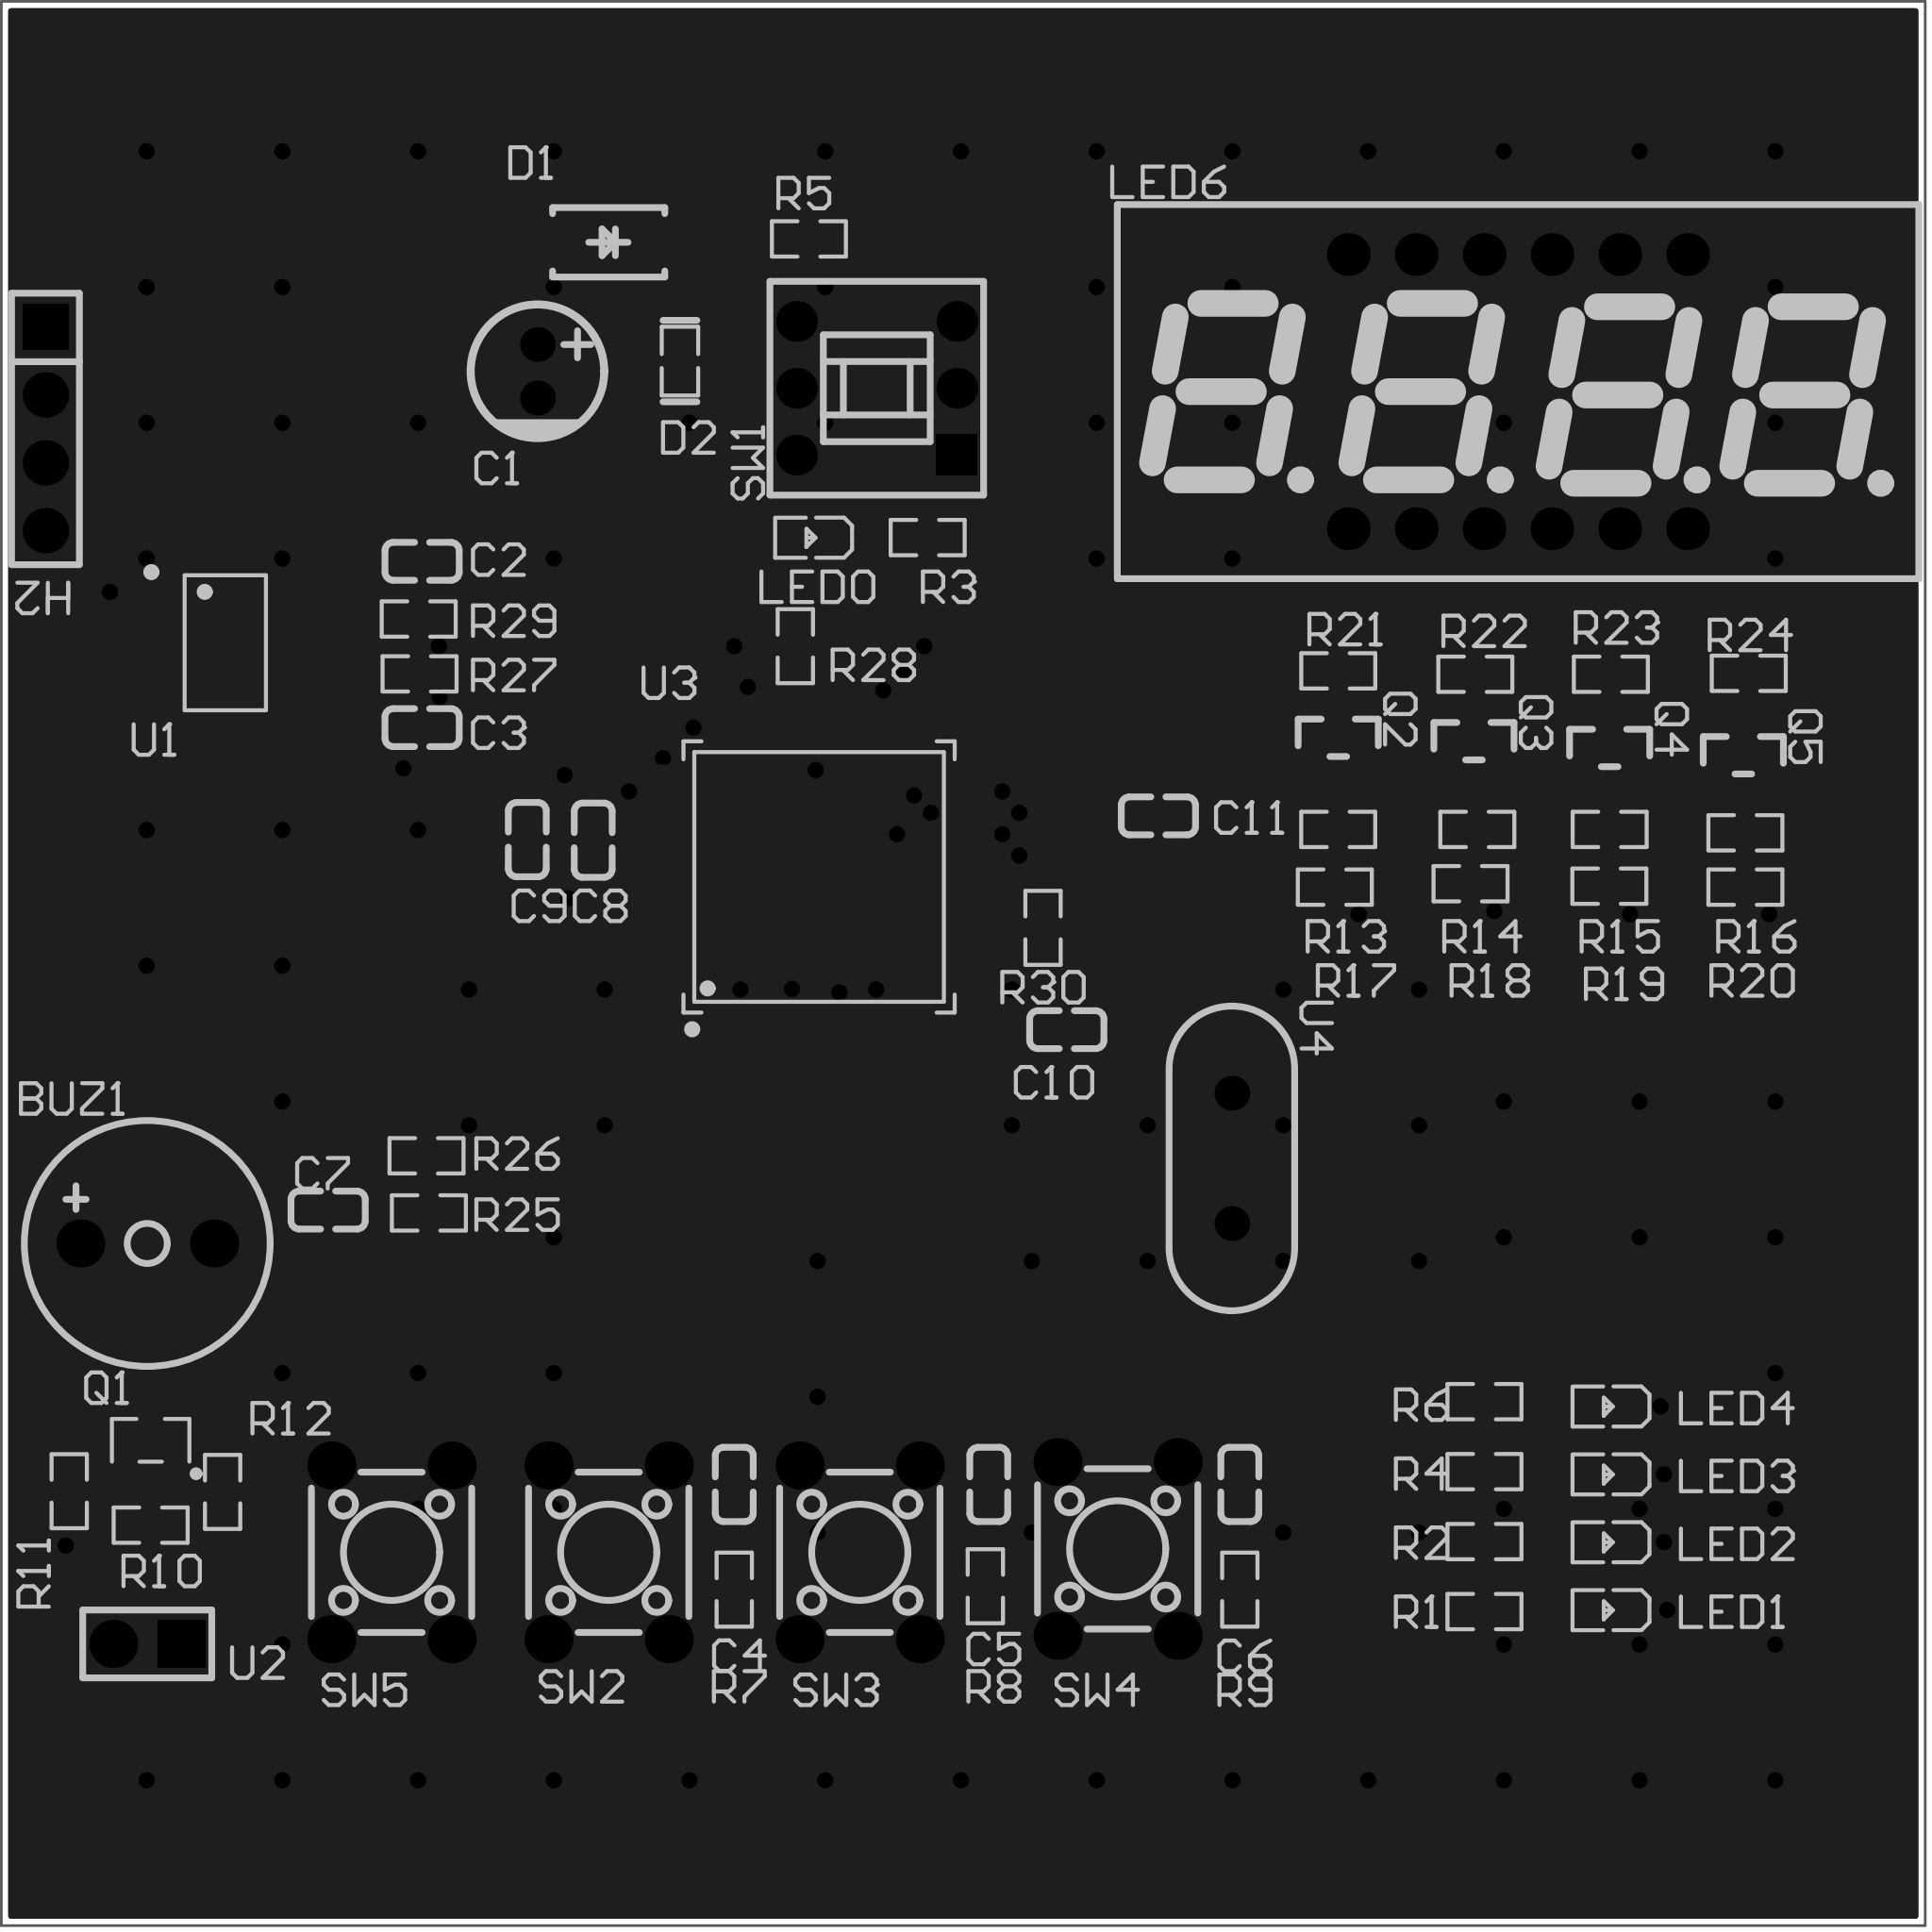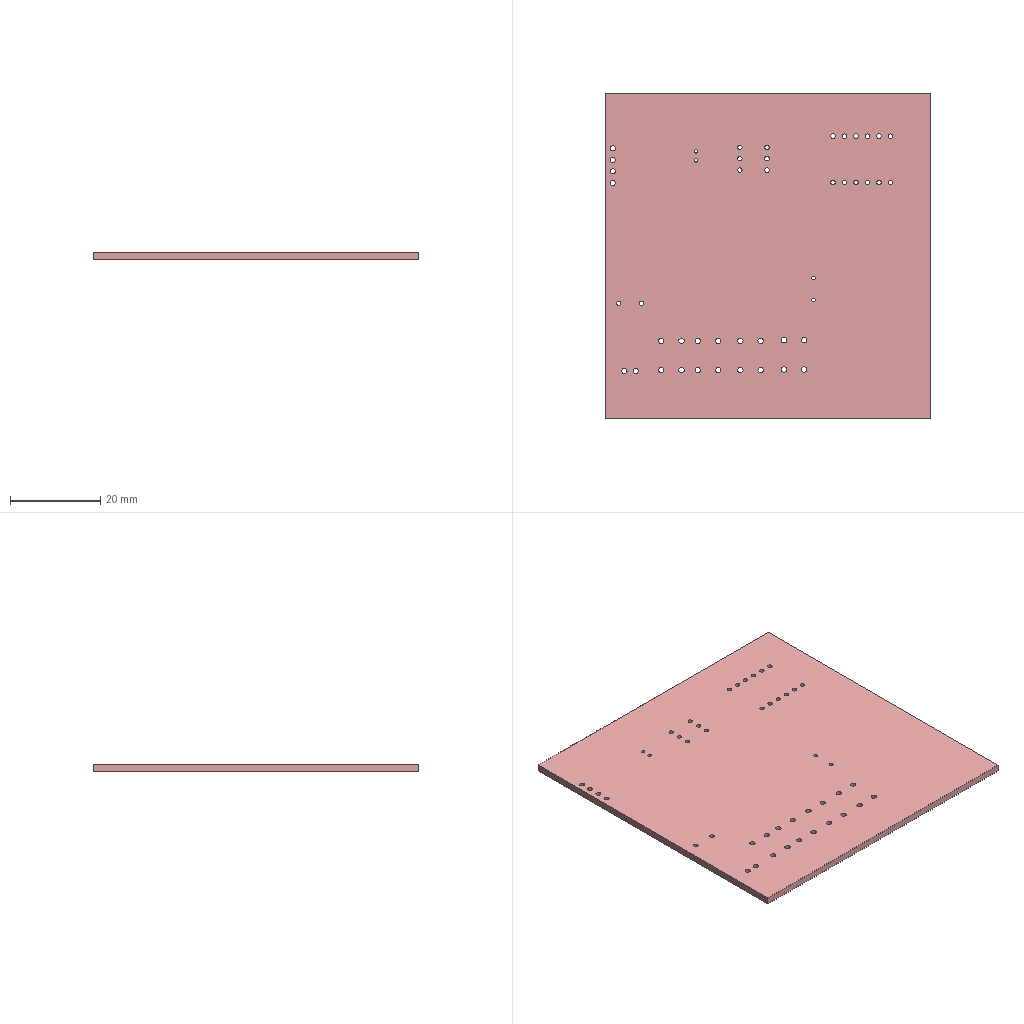Circuit board layout | Altium Designer | box 72 x 72 x 1.6 mm
Layer stack:
# Altium Designer layer stack of  (unit mm; dielectric type: 0 none, 1 core, 2 prepreg, 3 surface material)
index,name,kind,layer,copper_thickness_mm,dielectric_type,dielectric_thickness_mm,dielectric_material,dielectric_constant
0,Top Paste Mask Layer,other,,,,,,
1,Top Silkscreen Layer,other,,,,,,
2,Top Solder Mask Layer,dielectric,,,3,0.01,,3.3
3,Top Layer,copper,Top Layer,0.035,,,,
4,Dielectric1,dielectric,,,3,1.51,FR4,4.5
5,Bottom Layer,copper,Bottom Layer,0.035,,,,
6,Bottom Solder Mask Layer,dielectric,,,3,0.01,,3.3
7,Bottom Silkscreen Layer,other,,,,,,
8,Bottom Paste Mask Layer,other,,,,,,
# drill layer pairs: low layer,high layer
drill_pair,Top Layer,Bottom Layer
Part placement:
Designator,Comment,Layer,Footprint,Center-X(mm),Center-Y(mm),Rotation
BUZ1,SUN-09055-3,TopLayer,BUZ-TH_BD9.0-P5.00-D0.6-FD,95.631,116.713,0
C1,100uF,TopLayer,CAP-TH_BD5.0-P2.00-D0.8-FD,110.236,149.352,270
C2,100nF,TopLayer,C0603,105.918,142.24,0
C3,100nF,TopLayer,C0603,105.918,136.017,0
C4,100nF,TopLayer,C0603,117.602,107.696,90
C5,100nF,TopLayer,C0603,127.127,107.696,90
C6,100nF,TopLayer,C0603,136.525,107.696,90
C7,10uF,TopLayer,C0603,102.401,117.962,180
C8,100nF,TopLayer,C0603,112.323,131.805,270
C9,10uF,TopLayer,C0603,109.855,131.826,270
C10,47pF,TopLayer,C0603,130.048,124.714,0
C11,47pF,TopLayer,C0603,133.477,132.715,180
D1,SS14,TopLayer,SMA_L4.2-W2.6-LS5.0-RD_1,112.903,154.178,180
D2,0603ESDA-05N,TopLayer,D0603-BI,115.57,149.733,90
H2,PZ254V-11-04P,TopLayer,HDR-TH_4P-P2.54-V-M,91.821,147.193,270
LED0,NCD0603R1,TopLayer,LED0603-RD_RED,120.523,143.129,180
LED1,NCD0603R1,TopLayer,LED0603-RD_RED,150.368,102.997,180
LED2,NCD0603R1,TopLayer,LED0603-RD_RED,150.368,105.537,180
LED3,NCD0603R1,TopLayer,LED0603-RD_RED,150.368,108.077,180
LED4,NCD0603R1,TopLayer,LED0603-RD_RED,150.368,110.617,180
LED6,SR410361N,TopLayer,LED-SEG-TH_12P-L30.0-W14.0-P2.54-S10.26-BL,146.939,148.59,0
Q1,2N3906S-RTK/P,TopLayer,SOT-23-3_L2.9-W1.6-P1.90-LS2.8-TR-CW,95.758,109.347,270
Q2,AO3401A,TopLayer,SOT-23_L2.9-W1.3-P1.90-LS2.4-BR,140.208,135.636,270
Q3,AO3401A,TopLayer,SOT-23_L2.9-W1.3-P1.90-LS2.4-BR,145.288,135.509,270
Q4,AO3401A,TopLayer,SOT-23_L2.9-W1.3-P1.90-LS2.4-BR,150.368,135.255,270
Q5,AO3401A,TopLayer,SOT-23_L2.9-W1.3-P1.90-LS2.4-BR,155.371,134.982,270
R1,4.7kΩ,TopLayer,R0603,145.682,102.937,0
R2,4.7kΩ,TopLayer,R0603,145.682,105.556,0
R3,4.7kΩ,TopLayer,R0603,124.841,143.129,180
R4,4.7kΩ,TopLayer,R0603,145.682,108.174,0
R5,2kΩ,TopLayer,R0603,120.396,154.305,180
R6,4.7kΩ,TopLayer,R0603,145.682,110.793,0
R7,10kΩ,TopLayer,R0603,117.602,103.759,270
R8,10kΩ,TopLayer,R0603,127,103.886,270
R9,10kΩ,TopLayer,R0603,136.525,103.759,270
R10,10kΩ,TopLayer,R0603,95.758,106.172,0
R11,1kΩ,TopLayer,R0603,92.71,107.442,90
R12,10Ω,TopLayer,R0603,98.452,107.416,90
R13,10kΩ,TopLayer,R0603,140.208,132.207,0
R14,10kΩ,TopLayer,R0603,145.415,132.207,0
R15,10kΩ,TopLayer,R0603,150.368,132.207,0
R16,10kΩ,TopLayer,R0603,155.448,132.08,0
R17,1kΩ,TopLayer,R0603,140.081,130.048,180
R18,1kΩ,TopLayer,R0603,145.161,130.175,180
R19,1kΩ,TopLayer,R0603,150.357,130.083,0
R20,1kΩ,TopLayer,R0603,155.448,130.048,0
R21,47Ω,TopLayer,R0603,140.21,138.141,180
R22,47Ω,TopLayer,R0603,145.339,138.014,0
R23,47Ω,TopLayer,R0603,150.413,138.014,180
R24,47Ω,TopLayer,R0603,155.575,138.049,0
R25,100Ω,TopLayer,R0603,106.172,117.856,0
R26,10kΩ,TopLayer,R0603,106.084,119.994,0
R27,1kΩ,TopLayer,R0603,105.823,138.028,0
R28,10kΩ,TopLayer,R0603,119.888,139.065,90
R29,1kΩ,TopLayer,R0603,105.791,140.081,0
R30,1MΩ,TopLayer,R0603,129.159,128.524,270
SW1,XKB8080-Z,TopLayer,SW-TH_6P-L8.0-W8.0-P2.50,122.936,148.717,90
SW2,TS-1095-A5B2-D1,TopLayer,SW-TH_4P-L6.0-W6.0-P4.50-LS6.5,112.903,105.156,270
SW3,TS-1095-A5B2-D1,TopLayer,SW-TH_4P-L6.0-W6.0-P4.50-LS6.5,122.301,105.156,270
SW4,TS-1095-A5B2-D1,TopLayer,SW-TH_4P-L6.0-W6.0-P4.50-LS6.5,131.953,105.283,270
SW5,TS-1095-A5B2-D1,TopLayer,SW-TH_4P-L6.0-W6.0-P4.50-LS6.5,104.775,105.156,90
U1,CH340N,TopLayer,SOP-8_L5.0-W4.0-P1.27-LS6.0-BL,98.552,139.192,270
U2,54102-T0600LF,TopLayer,HDR-TH_2P-P2.54-V-M-R2-C1-S2.54,95.631,101.727,90
U3,STC89C52RC-40I-LQFP44,TopLayer,LQFP-44_L10.0-W10.0-P0.80-LS12.0-BL,120.777,130.429,0
U4,12MHz,TopLayer,HC-49S_L11.4-W4.7-P4.88-D0.4,136.228,119.896,270
Pad and via stacks:
# Altium Designer via and pad stacks of  (unit mm). Each distinct definition once, with the count of objects using it.
# via: kind,start_layer,end_layer,hole_mm,diameter_mm,mode(0 simple;1 top-mid-bottom;2 full stack),diameter_per_layer,count,example_net
# pad: kind,layer,hole_mm,hole_type(0 round;1 square;2 slot),plating,top_size,top_shape(1 round;2 rect;3 octagon;9 rounded rect),mid_size,bottom_size,mode,footprint,size_per_layer,count,example
pad,Multi-Layer,1,0,plated,1.8x1.8,1,1.8x1.8,1.8x1.8,0,BUZ-TH_BD9.0-P5.00-D0.6-FD,,2,BUZ1.1
pad,Multi-Layer,0.8,0,plated,1.3x1.3,1,1.3x1.3,1.3x1.3,0,CAP-TH_BD5.0-P2.00-D0.8-FD,,2,C1.1
pad,Multi-Layer,1.1,0,plated,1.7x1.7,2,1.7x1.7,1.7x1.7,0,HDR-TH_4P-P2.54-V-M,,1,H2.1
pad,Multi-Layer,1.1,0,plated,1.7x1.7,1,1.7x1.7,1.7x1.7,0,HDR-TH_4P-P2.54-V-M,,3,H2.2
pad,Multi-Layer,1,0,plated,1.6x1.6,1,1.6x1.6,1.6x1.6,0,LED-SEG-TH_12P-L30.0-W14.0-P2.54-S10.26-BL,,12,LED6.12
pad,Multi-Layer,1,0,plated,1.524x1.524,1,1.524x1.524,1.524x1.524,0,SW-TH_6P-L8.0-W8.0-P2.50,,5,SW1.3
pad,Multi-Layer,1,0,plated,1.524x1.524,2,1.524x1.524,1.524x1.524,0,SW-TH_6P-L8.0-W8.0-P2.50,,1,SW1.1
pad,Multi-Layer,1.2,0,plated,1.8x1.8,1,1.8x1.8,1.8x1.8,0,SW-TH_4P-L6.0-W6.0-P4.50-LS6.5,,16,SW2.1
pad,Multi-Layer,1.2,0,plated,1.8x1.8,1,1.8x1.8,1.8x1.8,0,HDR-TH_2P-P2.54-V-M-R2-C1-S2.54,,1,U2.2
pad,Multi-Layer,1.2,0,plated,1.8x1.8,2,1.8x1.8,1.8x1.8,0,HDR-TH_2P-P2.54-V-M-R2-C1-S2.54,,1,U2.1
pad,Multi-Layer,0.8,0,plated,1.3x1.3,1,1.3x1.3,1.3x1.3,0,HC-49S_L11.4-W4.7-P4.88-D0.4,,2,U4.2
pad,Top Layer,0,0,plated,0.8x0.9,2,0.8x0.9,0.8x0.9,0,C0603,,20,C2.2
pad,Top Layer,0,0,plated,1.52x1.68,2,1.52x1.68,1.52x1.68,0,SMA_L4.2-W2.6-LS5.0-RD_1,,2,D1.2
pad,Top Layer,0,0,plated,0.8732x0.9072,2,0.8732x0.9072,0.8732x0.9072,0,D0603-BI,,2,D2.2
pad,Top Layer,0,0,plated,0.8x0.8,2,0.8x0.8,0.8x0.8,0,LED0603-RD_RED,,10,LED0.1
pad,Top Layer,0,0,plated,0.7x1.25,2,0.7x1.25,0.7x1.25,0,SOT-23-3_L2.9-W1.6-P1.90-LS2.8-TR-CW,,3,Q1.2
pad,Top Layer,0,0,plated,1x0.8,2,1x0.8,1x0.8,0,SOT-23_L2.9-W1.3-P1.90-LS2.4-BR,,12,Q2.2
pad,Top Layer,0,0,plated,0.8065x0.864,2,0.8065x0.864,0.8065x0.864,0,R0603,,60,R1.2
pad,Top Layer,0,0,plated,0.574x2.035,1,0.574x2.035,0.574x2.035,0,SOP-8_L5.0-W4.0-P1.27-LS6.0-BL,,8,U1.1
pad,Top Layer,0,0,plated,0.42x1.67,1,0.42x1.67,0.42x1.67,0,LQFP-44_L10.0-W10.0-P0.80-LS12.0-BL,,22,U3.1
pad,Top Layer,0,0,plated,1.67x0.42,1,1.67x0.42,1.67x0.42,0,LQFP-44_L10.0-W10.0-P0.80-LS12.0-BL,,22,U3.12
via,Top Layer,Bottom Layer,0.3048,0.61,0,,129,SEGA
Copper pours:
name,layer,net,type(0 solid;1 hatched;2 none)
Bottom Layer-GND,Bottom Layer,GND,0
Top Layer-GND,Top Layer,GND,0
Design rules, without the lines most boards share:
# Altium Designer design rules of  (exported by Altium Designer, unit mm)
# columns: name | kind | enabled | priority | scope1 | scope2 | descriptor | typed fields (field=value)
creepage | 65 | enabled | 1 | All | All | Creepage Distance Constraint =(0mil) (All),(All) |